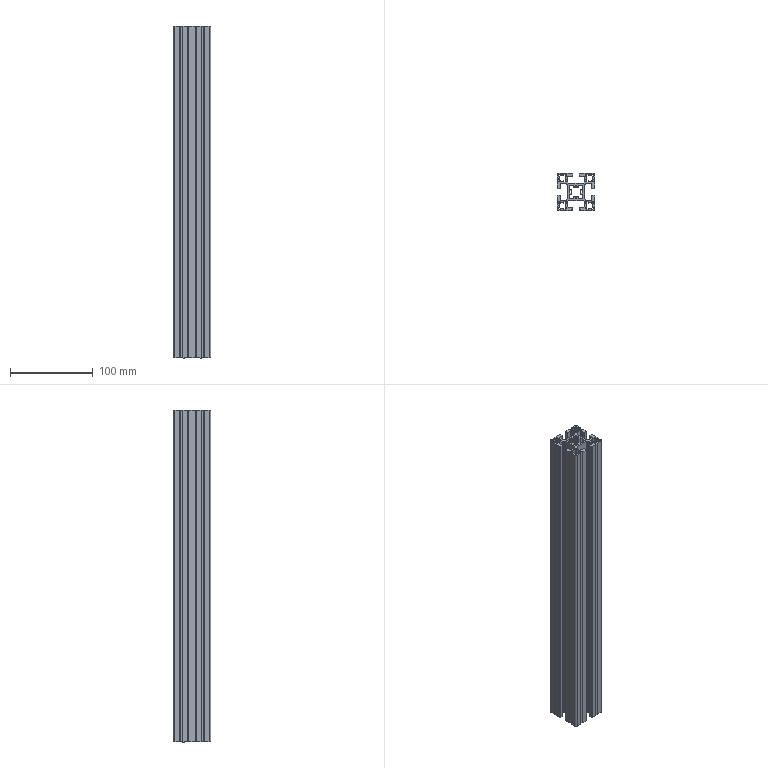Part | STEP file | 4545-400 Al (rack asm 1) | 1 solid | 262 faces | box 45 x 45 x 400 mm | volume 277539 mm3 | plane 186 | cylinder 76 | commonest cylinder face diameters 2 x44 8 x20 12 x8 4 x4